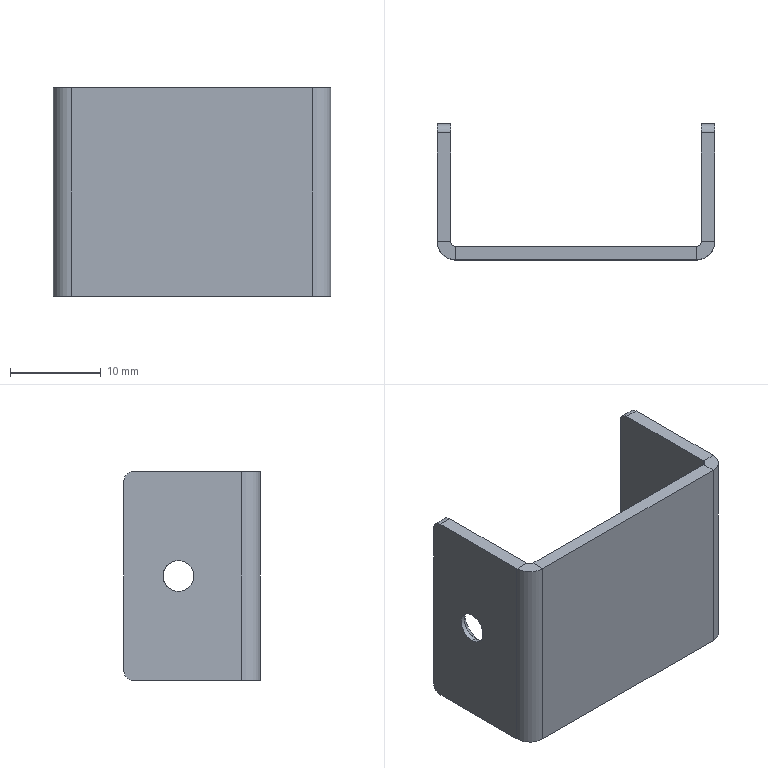Part | NX | features solid 2 | 1 solid | 34 faces | box 30.6 x 15 x 23 mm | volume 1909 mm3 | plane 18 | cylinder 12 | cone 4 | commonest cylinder face diameters 2 x4 3.4 x4 1 x2 4 x2
STEP:
#1=CARTESIAN_POINT('',(15.6,17.1,-1064.01));
#2=VERTEX_POINT('',#1);
#3=CARTESIAN_POINT('',(15.6,17.1,-1085.01));
#4=VERTEX_POINT('',#3);
#5=CARTESIAN_POINT('',(15.6,17.1,-1064.01));
#6=DIRECTION('',(0.,0.,-1.));
#7=VECTOR('',#6,1000.);
#8=LINE('',#5,#7);
#9=EDGE_CURVE('',#2,#4,#8,.T.);
#10=ORIENTED_EDGE('',*,*,#9,.F.);
#11=CARTESIAN_POINT('',(15.6,16.1,-1063.01));
#12=VERTEX_POINT('',#11);
#13=CARTESIAN_POINT('',(15.6,16.1,-1064.01));
#14=DIRECTION('',(-1.,0.,0.));
#15=DIRECTION('',(0.,0.,1.));
#16=AXIS2_PLACEMENT_3D('',#13,#14,#15);
#17=CIRCLE('',#16,1.);
#18=EDGE_CURVE('',#12,#2,#17,.T.);
#19=ORIENTED_EDGE('',*,*,#18,.F.);
#20=CARTESIAN_POINT('',(15.6,4.1,-1063.01));
#21=VERTEX_POINT('',#20);
#22=CARTESIAN_POINT('',(15.6,16.1,-1063.01));
#23=DIRECTION('',(0.,-1.,0.));
#24=VECTOR('',#23,1000.);
#25=LINE('',#22,#24);
#26=EDGE_CURVE('',#12,#21,#25,.T.);
#27=ORIENTED_EDGE('',*,*,#26,.T.);
#28=CARTESIAN_POINT('',(15.6,4.1,-1086.01));
#29=VERTEX_POINT('',#28);
#30=CARTESIAN_POINT('',(15.6,4.1,-1063.01));
#31=DIRECTION('',(0.,0.,-1.));
#32=VECTOR('',#31,1000.);
#33=LINE('',#30,#32);
#34=EDGE_CURVE('',#21,#29,#33,.T.);
#35=ORIENTED_EDGE('',*,*,#34,.T.);
#36=CARTESIAN_POINT('',(15.6,16.1,-1086.01));
#37=VERTEX_POINT('',#36);
#38=CARTESIAN_POINT('',(15.6,16.1,-1086.01));
#39=DIRECTION('',(0.,-1.,0.));
#40=VECTOR('',#39,1000.);
#41=LINE('',#38,#40);
#42=EDGE_CURVE('',#37,#29,#41,.T.);
#43=ORIENTED_EDGE('',*,*,#42,.F.);
#44=CARTESIAN_POINT('',(15.6,16.1,-1085.01));
#45=DIRECTION('',(-1.,0.,0.));
#46=DIRECTION('',(0.,1.,0.));
#47=AXIS2_PLACEMENT_3D('',#44,#45,#46);
#48=CIRCLE('',#47,1.);
#49=EDGE_CURVE('',#4,#37,#48,.T.);
#50=ORIENTED_EDGE('',*,*,#49,.F.);
#51=EDGE_LOOP('',(#10,#19,#27,#35,#43,#50));
#52=FACE_BOUND('',#51,.T.);
#53=CARTESIAN_POINT('',(15.6,11.1,-1076.21));
#54=VERTEX_POINT('',#53);
#55=CARTESIAN_POINT('',(15.6,11.1,-1072.81));
#56=VERTEX_POINT('',#55);
#57=CARTESIAN_POINT('',(15.6,11.1,-1074.51));
#58=DIRECTION('',(1.,0.,0.));
#59=DIRECTION('',(0.,0.,-1.));
#60=AXIS2_PLACEMENT_3D('',#57,#58,#59);
#61=CIRCLE('',#60,1.7);
#62=EDGE_CURVE('',#54,#56,#61,.T.);
#63=ORIENTED_EDGE('',*,*,#62,.F.);
#64=CARTESIAN_POINT('',(15.6,11.1,-1074.51));
#65=DIRECTION('',(1.,0.,0.));
#66=DIRECTION('',(0.,0.,1.));
#67=AXIS2_PLACEMENT_3D('',#64,#65,#66);
#68=CIRCLE('',#67,1.7);
#69=EDGE_CURVE('',#56,#54,#68,.T.);
#70=ORIENTED_EDGE('',*,*,#69,.F.);
#71=EDGE_LOOP('',(#63,#70));
#72=FACE_BOUND('',#71,.T.);
#73=CARTESIAN_POINT('',(15.6,2.1,-1086.01));
#74=DIRECTION('',(1.,0.,0.));
#75=DIRECTION('',(0.,-1.,0.));
#76=AXIS2_PLACEMENT_3D('',#73,#74,#75);
#77=PLANE('',#76);
#78=ADVANCED_FACE('',(#52,#72),#77,.T.);
#79=CARTESIAN_POINT('',(14.1,16.1,-1086.01));
#80=VERTEX_POINT('',#79);
#81=CARTESIAN_POINT('',(14.1,16.1,-1086.01));
#82=DIRECTION('',(1.,0.,0.));
#83=VECTOR('',#82,1000.);
#84=LINE('',#81,#83);
#85=EDGE_CURVE('',#80,#37,#84,.T.);
#86=ORIENTED_EDGE('',*,*,#85,.F.);
#87=CARTESIAN_POINT('',(14.1,17.1,-1085.01));
#88=VERTEX_POINT('',#87);
#89=CARTESIAN_POINT('',(14.1,16.1,-1085.01));
#90=DIRECTION('',(1.,0.,0.));
#91=DIRECTION('',(0.,0.,-1.));
#92=AXIS2_PLACEMENT_3D('',#89,#90,#91);
#93=CIRCLE('',#92,1.);
#94=EDGE_CURVE('',#80,#88,#93,.T.);
#95=ORIENTED_EDGE('',*,*,#94,.T.);
#96=CARTESIAN_POINT('',(15.6,17.1,-1085.01));
#97=DIRECTION('',(-1.,0.,0.));
#98=VECTOR('',#97,1000.);
#99=LINE('',#96,#98);
#100=EDGE_CURVE('',#4,#88,#99,.T.);
#101=ORIENTED_EDGE('',*,*,#100,.F.);
#102=ORIENTED_EDGE('',*,*,#49,.T.);
#103=EDGE_LOOP('',(#86,#95,#101,#102));
#104=FACE_BOUND('',#103,.T.);
#105=CARTESIAN_POINT('',(-54.89,16.1,-1085.01));
#106=DIRECTION('',(1.,0.,0.));
#107=DIRECTION('',(0.,0.,1.));
#108=AXIS2_PLACEMENT_3D('',#105,#106,#107);
#109=CYLINDRICAL_SURFACE('',#108,1.);
#110=ADVANCED_FACE('',(#104),#109,.T.);
#111=CARTESIAN_POINT('',(14.1,17.1,-1064.01));
#112=VERTEX_POINT('',#111);
#113=CARTESIAN_POINT('',(14.1,17.1,-1064.01));
#114=DIRECTION('',(0.,0.,-1.));
#115=VECTOR('',#114,1000.);
#116=LINE('',#113,#115);
#117=EDGE_CURVE('',#112,#88,#116,.T.);
#118=ORIENTED_EDGE('',*,*,#117,.F.);
#119=CARTESIAN_POINT('',(14.1,17.1,-1064.01));
#120=DIRECTION('',(1.,0.,0.));
#121=VECTOR('',#120,1000.);
#122=LINE('',#119,#121);
#123=EDGE_CURVE('',#112,#2,#122,.T.);
#124=ORIENTED_EDGE('',*,*,#123,.T.);
#125=ORIENTED_EDGE('',*,*,#9,.T.);
#126=ORIENTED_EDGE('',*,*,#100,.T.);
#127=EDGE_LOOP('',(#118,#124,#125,#126));
#128=FACE_BOUND('',#127,.T.);
#129=CARTESIAN_POINT('',(14.85,17.1,-1074.51));
#130=DIRECTION('',(0.,1.,0.));
#131=DIRECTION('',(0.,0.,-1.));
#132=AXIS2_PLACEMENT_3D('',#129,#130,#131);
#133=PLANE('',#132);
#134=ADVANCED_FACE('',(#128),#133,.T.);
#135=ORIENTED_EDGE('',*,*,#123,.F.);
#136=CARTESIAN_POINT('',(14.1,16.1,-1063.01));
#137=VERTEX_POINT('',#136);
#138=CARTESIAN_POINT('',(14.1,16.1,-1064.01));
#139=DIRECTION('',(1.,0.,0.));
#140=DIRECTION('',(0.,1.,0.));
#141=AXIS2_PLACEMENT_3D('',#138,#139,#140);
#142=CIRCLE('',#141,1.);
#143=EDGE_CURVE('',#112,#137,#142,.T.);
#144=ORIENTED_EDGE('',*,*,#143,.T.);
#145=CARTESIAN_POINT('',(15.6,16.1,-1063.01));
#146=DIRECTION('',(-1.,0.,0.));
#147=VECTOR('',#146,1000.);
#148=LINE('',#145,#147);
#149=EDGE_CURVE('',#12,#137,#148,.T.);
#150=ORIENTED_EDGE('',*,*,#149,.F.);
#151=ORIENTED_EDGE('',*,*,#18,.T.);
#152=EDGE_LOOP('',(#135,#144,#150,#151));
#153=FACE_BOUND('',#152,.T.);
#154=CARTESIAN_POINT('',(-54.259,16.1,-1064.01));
#155=DIRECTION('',(1.,0.,0.));
#156=DIRECTION('',(0.,-1.,0.));
#157=AXIS2_PLACEMENT_3D('',#154,#155,#156);
#158=CYLINDRICAL_SURFACE('',#157,1.);
#159=ADVANCED_FACE('',(#153),#158,.T.);
#160=CARTESIAN_POINT('',(14.1,4.1,-1063.01));
#161=VERTEX_POINT('',#160);
#162=CARTESIAN_POINT('',(14.1,16.1,-1063.01));
#163=DIRECTION('',(0.,-1.,0.));
#164=VECTOR('',#163,1000.);
#165=LINE('',#162,#164);
#166=EDGE_CURVE('',#137,#161,#165,.T.);
#167=ORIENTED_EDGE('',*,*,#166,.T.);
#168=CARTESIAN_POINT('',(14.1,4.1,-1063.01));
#169=DIRECTION('',(1.,0.,0.));
#170=VECTOR('',#169,1000.);
#171=LINE('',#168,#170);
#172=EDGE_CURVE('',#161,#21,#171,.T.);
#173=ORIENTED_EDGE('',*,*,#172,.T.);
#174=ORIENTED_EDGE('',*,*,#26,.F.);
#175=ORIENTED_EDGE('',*,*,#149,.T.);
#176=EDGE_LOOP('',(#167,#173,#174,#175));
#177=FACE_BOUND('',#176,.T.);
#178=CARTESIAN_POINT('',(14.85,9.975,-1063.01));
#179=DIRECTION('',(0.,0.,-1.));
#180=DIRECTION('',(0.,-1.,0.));
#181=AXIS2_PLACEMENT_3D('',#178,#179,#180);
#182=PLANE('',#181);
#183=ADVANCED_FACE('',(#177),#182,.F.);
#184=ORIENTED_EDGE('',*,*,#172,.F.);
#185=CARTESIAN_POINT('',(13.6,3.6,-1063.01));
#186=VERTEX_POINT('',#185);
#187=CARTESIAN_POINT('',(13.6,4.1,-1063.01));
#188=DIRECTION('',(0.,0.,1.));
#189=DIRECTION('',(0.,-1.,0.));
#190=AXIS2_PLACEMENT_3D('',#187,#188,#189);
#191=CIRCLE('',#190,0.5);
#192=EDGE_CURVE('',#186,#161,#191,.T.);
#193=ORIENTED_EDGE('',*,*,#192,.F.);
#194=CARTESIAN_POINT('',(13.6,2.1,-1063.01));
#195=VERTEX_POINT('',#194);
#196=CARTESIAN_POINT('',(13.6,3.6,-1063.01));
#197=DIRECTION('',(0.,-1.,0.));
#198=VECTOR('',#197,1000.);
#199=LINE('',#196,#198);
#200=EDGE_CURVE('',#186,#195,#199,.T.);
#201=ORIENTED_EDGE('',*,*,#200,.T.);
#202=CARTESIAN_POINT('',(13.6,4.1,-1063.01));
#203=DIRECTION('',(0.,0.,-1.));
#204=DIRECTION('',(1.,0.,0.));
#205=AXIS2_PLACEMENT_3D('',#202,#203,#204);
#206=CIRCLE('',#205,2.);
#207=EDGE_CURVE('',#21,#195,#206,.T.);
#208=ORIENTED_EDGE('',*,*,#207,.F.);
#209=EDGE_LOOP('',(#184,#193,#201,#208));
#210=FACE_BOUND('',#209,.T.);
#211=CARTESIAN_POINT('',(14.484,3.216,-1063.01));
#212=DIRECTION('',(0.,0.,-1.));
#213=DIRECTION('',(-1.,0.,0.));
#214=AXIS2_PLACEMENT_3D('',#211,#212,#213);
#215=PLANE('',#214);
#216=ADVANCED_FACE('',(#210),#215,.F.);
#217=CARTESIAN_POINT('',(13.6,2.1,-1086.01));
#218=VERTEX_POINT('',#217);
#219=CARTESIAN_POINT('',(13.6,4.1,-1086.01));
#220=DIRECTION('',(0.,0.,1.));
#221=DIRECTION('',(0.,-1.,0.));
#222=AXIS2_PLACEMENT_3D('',#219,#220,#221);
#223=CIRCLE('',#222,2.);
#224=EDGE_CURVE('',#218,#29,#223,.T.);
#225=ORIENTED_EDGE('',*,*,#224,.T.);
#226=ORIENTED_EDGE('',*,*,#34,.F.);
#227=ORIENTED_EDGE('',*,*,#207,.T.);
#228=CARTESIAN_POINT('',(13.6,2.1,-1086.01));
#229=DIRECTION('',(0.,0.,1.));
#230=VECTOR('',#229,1000.);
#231=LINE('',#228,#230);
#232=EDGE_CURVE('',#218,#195,#231,.T.);
#233=ORIENTED_EDGE('',*,*,#232,.F.);
#234=EDGE_LOOP('',(#225,#226,#227,#233));
#235=FACE_BOUND('',#234,.T.);
#236=CARTESIAN_POINT('',(13.6,4.1,-1019.945));
#237=DIRECTION('',(0.,0.,-1.));
#238=DIRECTION('',(-1.,0.,0.));
#239=AXIS2_PLACEMENT_3D('',#236,#237,#238);
#240=CYLINDRICAL_SURFACE('',#239,2.);
#241=ADVANCED_FACE('',(#235),#240,.T.);
#242=CARTESIAN_POINT('',(-13.,2.1,-1063.01));
#243=VERTEX_POINT('',#242);
#244=CARTESIAN_POINT('',(13.6,2.1,-1063.01));
#245=DIRECTION('',(-1.,0.,0.));
#246=VECTOR('',#245,1000.);
#247=LINE('',#244,#246);
#248=EDGE_CURVE('',#195,#243,#247,.T.);
#249=ORIENTED_EDGE('',*,*,#248,.T.);
#250=CARTESIAN_POINT('',(-13.,2.1,-1086.01));
#251=VERTEX_POINT('',#250);
#252=CARTESIAN_POINT('',(-13.,2.1,-1063.01));
#253=DIRECTION('',(0.,0.,-1.));
#254=VECTOR('',#253,1000.);
#255=LINE('',#252,#254);
#256=EDGE_CURVE('',#243,#251,#255,.T.);
#257=ORIENTED_EDGE('',*,*,#256,.T.);
#258=CARTESIAN_POINT('',(13.6,2.1,-1086.01));
#259=DIRECTION('',(-1.,0.,0.));
#260=VECTOR('',#259,1000.);
#261=LINE('',#258,#260);
#262=EDGE_CURVE('',#218,#251,#261,.T.);
#263=ORIENTED_EDGE('',*,*,#262,.F.);
#264=ORIENTED_EDGE('',*,*,#232,.T.);
#265=EDGE_LOOP('',(#249,#257,#263,#264));
#266=FACE_BOUND('',#265,.T.);
#267=CARTESIAN_POINT('',(-15.,2.1,-1086.01));
#268=DIRECTION('',(0.,-1.,0.));
#269=DIRECTION('',(-1.,0.,0.));
#270=AXIS2_PLACEMENT_3D('',#267,#268,#269);
#271=PLANE('',#270);
#272=ADVANCED_FACE('',(#266),#271,.T.);
#273=ORIENTED_EDGE('',*,*,#262,.T.);
#274=CARTESIAN_POINT('',(-13.,3.6,-1086.01));
#275=VERTEX_POINT('',#274);
#276=CARTESIAN_POINT('',(-13.,3.6,-1086.01));
#277=DIRECTION('',(0.,-1.,0.));
#278=VECTOR('',#277,1000.);
#279=LINE('',#276,#278);
#280=EDGE_CURVE('',#275,#251,#279,.T.);
#281=ORIENTED_EDGE('',*,*,#280,.F.);
#282=CARTESIAN_POINT('',(13.6,3.6,-1086.01));
#283=VERTEX_POINT('',#282);
#284=CARTESIAN_POINT('',(13.6,3.6,-1086.01));
#285=DIRECTION('',(-1.,0.,0.));
#286=VECTOR('',#285,1000.);
#287=LINE('',#284,#286);
#288=EDGE_CURVE('',#283,#275,#287,.T.);
#289=ORIENTED_EDGE('',*,*,#288,.F.);
#290=CARTESIAN_POINT('',(13.6,3.6,-1086.01));
#291=DIRECTION('',(0.,-1.,0.));
#292=VECTOR('',#291,1000.);
#293=LINE('',#290,#292);
#294=EDGE_CURVE('',#283,#218,#293,.T.);
#295=ORIENTED_EDGE('',*,*,#294,.T.);
#296=EDGE_LOOP('',(#273,#281,#289,#295));
#297=FACE_BOUND('',#296,.T.);
#298=CARTESIAN_POINT('',(0.3,2.85,-1086.01));
#299=DIRECTION('',(0.,0.,-1.));
#300=DIRECTION('',(-1.,0.,0.));
#301=AXIS2_PLACEMENT_3D('',#298,#299,#300);
#302=PLANE('',#301);
#303=ADVANCED_FACE('',(#297),#302,.T.);
#304=ORIENTED_EDGE('',*,*,#294,.F.);
#305=CARTESIAN_POINT('',(14.1,4.1,-1086.01));
#306=VERTEX_POINT('',#305);
#307=CARTESIAN_POINT('',(13.6,4.1,-1086.01));
#308=DIRECTION('',(0.,0.,-1.));
#309=DIRECTION('',(1.,0.,0.));
#310=AXIS2_PLACEMENT_3D('',#307,#308,#309);
#311=CIRCLE('',#310,0.5);
#312=EDGE_CURVE('',#306,#283,#311,.T.);
#313=ORIENTED_EDGE('',*,*,#312,.F.);
#314=CARTESIAN_POINT('',(14.1,4.1,-1086.01));
#315=DIRECTION('',(1.,0.,0.));
#316=VECTOR('',#315,1000.);
#317=LINE('',#314,#316);
#318=EDGE_CURVE('',#306,#29,#317,.T.);
#319=ORIENTED_EDGE('',*,*,#318,.T.);
#320=ORIENTED_EDGE('',*,*,#224,.F.);
#321=EDGE_LOOP('',(#304,#313,#319,#320));
#322=FACE_BOUND('',#321,.T.);
#323=CARTESIAN_POINT('',(14.484,3.216,-1086.01));
#324=DIRECTION('',(0.,0.,1.));
#325=DIRECTION('',(0.,1.,0.));
#326=AXIS2_PLACEMENT_3D('',#323,#324,#325);
#327=PLANE('',#326);
#328=ADVANCED_FACE('',(#322),#327,.F.);
#329=ORIENTED_EDGE('',*,*,#42,.T.);
#330=ORIENTED_EDGE('',*,*,#318,.F.);
#331=CARTESIAN_POINT('',(14.1,16.1,-1086.01));
#332=DIRECTION('',(0.,-1.,0.));
#333=VECTOR('',#332,1000.);
#334=LINE('',#331,#333);
#335=EDGE_CURVE('',#80,#306,#334,.T.);
#336=ORIENTED_EDGE('',*,*,#335,.F.);
#337=ORIENTED_EDGE('',*,*,#85,.T.);
#338=EDGE_LOOP('',(#329,#330,#336,#337));
#339=FACE_BOUND('',#338,.T.);
#340=CARTESIAN_POINT('',(14.85,9.975,-1086.01));
#341=DIRECTION('',(0.,0.,-1.));
#342=DIRECTION('',(0.,-1.,0.));
#343=AXIS2_PLACEMENT_3D('',#340,#341,#342);
#344=PLANE('',#343);
#345=ADVANCED_FACE('',(#339),#344,.T.);
#346=ORIENTED_EDGE('',*,*,#335,.T.);
#347=CARTESIAN_POINT('',(14.1,4.1,-1086.01));
#348=DIRECTION('',(0.,0.,1.));
#349=VECTOR('',#348,1000.);
#350=LINE('',#347,#349);
#351=EDGE_CURVE('',#306,#161,#350,.T.);
#352=ORIENTED_EDGE('',*,*,#351,.T.);
#353=ORIENTED_EDGE('',*,*,#166,.F.);
#354=ORIENTED_EDGE('',*,*,#143,.F.);
#355=ORIENTED_EDGE('',*,*,#117,.T.);
#356=ORIENTED_EDGE('',*,*,#94,.F.);
#357=EDGE_LOOP('',(#346,#352,#353,#354,#355,#356));
#358=FACE_BOUND('',#357,.T.);
#359=CARTESIAN_POINT('',(14.1,8.4,-1074.51));
#360=VERTEX_POINT('',#359);
#361=CARTESIAN_POINT('',(14.1,11.1,-1071.81));
#362=VERTEX_POINT('',#361);
#363=CARTESIAN_POINT('',(14.1,11.1,-1074.51));
#364=DIRECTION('',(-1.,0.,0.));
#365=DIRECTION('',(0.,-1.,0.));
#366=AXIS2_PLACEMENT_3D('',#363,#364,#365);
#367=CIRCLE('',#366,2.7);
#368=EDGE_CURVE('',#360,#362,#367,.T.);
#369=ORIENTED_EDGE('',*,*,#368,.F.);
#370=CARTESIAN_POINT('',(14.1,11.1,-1077.21));
#371=VERTEX_POINT('',#370);
#372=CARTESIAN_POINT('',(14.1,11.1,-1074.51));
#373=DIRECTION('',(-1.,0.,0.));
#374=DIRECTION('',(0.,0.,-1.));
#375=AXIS2_PLACEMENT_3D('',#372,#373,#374);
#376=CIRCLE('',#375,2.7);
#377=EDGE_CURVE('',#371,#360,#376,.T.);
#378=ORIENTED_EDGE('',*,*,#377,.F.);
#379=CARTESIAN_POINT('',(14.1,13.8,-1074.51));
#380=VERTEX_POINT('',#379);
#381=CARTESIAN_POINT('',(14.1,11.1,-1074.51));
#382=DIRECTION('',(-1.,0.,0.));
#383=DIRECTION('',(0.,1.,0.));
#384=AXIS2_PLACEMENT_3D('',#381,#382,#383);
#385=CIRCLE('',#384,2.7);
#386=EDGE_CURVE('',#380,#371,#385,.T.);
#387=ORIENTED_EDGE('',*,*,#386,.F.);
#388=CARTESIAN_POINT('',(14.1,11.1,-1074.51));
#389=DIRECTION('',(-1.,0.,0.));
#390=DIRECTION('',(0.,0.,1.));
#391=AXIS2_PLACEMENT_3D('',#388,#389,#390);
#392=CIRCLE('',#391,2.7);
#393=EDGE_CURVE('',#362,#380,#392,.T.);
#394=ORIENTED_EDGE('',*,*,#393,.F.);
#395=EDGE_LOOP('',(#369,#378,#387,#394));
#396=FACE_BOUND('',#395,.T.);
#397=CARTESIAN_POINT('',(14.1,2.1,-1086.01));
#398=DIRECTION('',(1.,0.,0.));
#399=DIRECTION('',(0.,-1.,0.));
#400=AXIS2_PLACEMENT_3D('',#397,#398,#399);
#401=PLANE('',#400);
#402=ADVANCED_FACE('',(#358,#396),#401,.F.);
#403=ORIENTED_EDGE('',*,*,#192,.T.);
#404=ORIENTED_EDGE('',*,*,#351,.F.);
#405=ORIENTED_EDGE('',*,*,#312,.T.);
#406=CARTESIAN_POINT('',(13.6,3.6,-1063.01));
#407=DIRECTION('',(0.,0.,-1.));
#408=VECTOR('',#407,1000.);
#409=LINE('',#406,#408);
#410=EDGE_CURVE('',#186,#283,#409,.T.);
#411=ORIENTED_EDGE('',*,*,#410,.F.);
#412=EDGE_LOOP('',(#403,#404,#405,#411));
#413=FACE_BOUND('',#412,.T.);
#414=CARTESIAN_POINT('',(13.6,4.1,-1019.945));
#415=DIRECTION('',(0.,0.,-1.));
#416=DIRECTION('',(-1.,0.,0.));
#417=AXIS2_PLACEMENT_3D('',#414,#415,#416);
#418=CYLINDRICAL_SURFACE('',#417,0.5);
#419=ADVANCED_FACE('',(#413),#418,.F.);
#420=ORIENTED_EDGE('',*,*,#288,.T.);
#421=CARTESIAN_POINT('',(-13.,3.6,-1063.01));
#422=VERTEX_POINT('',#421);
#423=CARTESIAN_POINT('',(-13.,3.6,-1086.01));
#424=DIRECTION('',(0.,0.,1.));
#425=VECTOR('',#424,1000.);
#426=LINE('',#423,#425);
#427=EDGE_CURVE('',#275,#422,#426,.T.);
#428=ORIENTED_EDGE('',*,*,#427,.T.);
#429=CARTESIAN_POINT('',(13.6,3.6,-1063.01));
#430=DIRECTION('',(-1.,0.,0.));
#431=VECTOR('',#430,1000.);
#432=LINE('',#429,#431);
#433=EDGE_CURVE('',#186,#422,#432,.T.);
#434=ORIENTED_EDGE('',*,*,#433,.F.);
#435=ORIENTED_EDGE('',*,*,#410,.T.);
#436=EDGE_LOOP('',(#420,#428,#434,#435));
#437=FACE_BOUND('',#436,.T.);
#438=CARTESIAN_POINT('',(-15.,3.6,-1086.01));
#439=DIRECTION('',(0.,-1.,0.));
#440=DIRECTION('',(-1.,0.,0.));
#441=AXIS2_PLACEMENT_3D('',#438,#439,#440);
#442=PLANE('',#441);
#443=ADVANCED_FACE('',(#437),#442,.F.);
#444=ORIENTED_EDGE('',*,*,#248,.F.);
#445=ORIENTED_EDGE('',*,*,#200,.F.);
#446=ORIENTED_EDGE('',*,*,#433,.T.);
#447=CARTESIAN_POINT('',(-13.,3.6,-1063.01));
#448=DIRECTION('',(0.,-1.,0.));
#449=VECTOR('',#448,1000.);
#450=LINE('',#447,#449);
#451=EDGE_CURVE('',#422,#243,#450,.T.);
#452=ORIENTED_EDGE('',*,*,#451,.T.);
#453=EDGE_LOOP('',(#444,#445,#446,#452));
#454=FACE_BOUND('',#453,.T.);
#455=CARTESIAN_POINT('',(0.3,2.85,-1063.01));
#456=DIRECTION('',(0.,0.,-1.));
#457=DIRECTION('',(-1.,0.,0.));
#458=AXIS2_PLACEMENT_3D('',#455,#456,#457);
#459=PLANE('',#458);
#460=ADVANCED_FACE('',(#454),#459,.F.);
#461=ORIENTED_EDGE('',*,*,#451,.F.);
#462=CARTESIAN_POINT('',(-13.5,4.1,-1063.01));
#463=VERTEX_POINT('',#462);
#464=CARTESIAN_POINT('',(-13.,4.1,-1063.01));
#465=DIRECTION('',(0.,0.,1.));
#466=DIRECTION('',(-1.,0.,0.));
#467=AXIS2_PLACEMENT_3D('',#464,#465,#466);
#468=CIRCLE('',#467,0.5);
#469=EDGE_CURVE('',#463,#422,#468,.T.);
#470=ORIENTED_EDGE('',*,*,#469,.F.);
#471=CARTESIAN_POINT('',(-15.,4.1,-1063.01));
#472=VERTEX_POINT('',#471);
#473=CARTESIAN_POINT('',(-13.5,4.1,-1063.01));
#474=DIRECTION('',(-1.,0.,0.));
#475=VECTOR('',#474,1000.);
#476=LINE('',#473,#475);
#477=EDGE_CURVE('',#463,#472,#476,.T.);
#478=ORIENTED_EDGE('',*,*,#477,.T.);
#479=CARTESIAN_POINT('',(-13.,4.1,-1063.01));
#480=DIRECTION('',(0.,0.,-1.));
#481=DIRECTION('',(0.,-1.,0.));
#482=AXIS2_PLACEMENT_3D('',#479,#480,#481);
#483=CIRCLE('',#482,2.);
#484=EDGE_CURVE('',#243,#472,#483,.T.);
#485=ORIENTED_EDGE('',*,*,#484,.F.);
#486=EDGE_LOOP('',(#461,#470,#478,#485));
#487=FACE_BOUND('',#486,.T.);
#488=CARTESIAN_POINT('',(-13.884,3.216,-1063.01));
#489=DIRECTION('',(0.,0.,-1.));
#490=DIRECTION('',(0.,1.,0.));
#491=AXIS2_PLACEMENT_3D('',#488,#489,#490);
#492=PLANE('',#491);
#493=ADVANCED_FACE('',(#487),#492,.F.);
#494=CARTESIAN_POINT('',(-15.,4.1,-1086.01));
#495=VERTEX_POINT('',#494);
#496=CARTESIAN_POINT('',(-13.,4.1,-1086.01));
#497=DIRECTION('',(0.,0.,1.));
#498=DIRECTION('',(-1.,0.,0.));
#499=AXIS2_PLACEMENT_3D('',#496,#497,#498);
#500=CIRCLE('',#499,2.);
#501=EDGE_CURVE('',#495,#251,#500,.T.);
#502=ORIENTED_EDGE('',*,*,#501,.T.);
#503=ORIENTED_EDGE('',*,*,#256,.F.);
#504=ORIENTED_EDGE('',*,*,#484,.T.);
#505=CARTESIAN_POINT('',(-15.,4.1,-1086.01));
#506=DIRECTION('',(0.,0.,1.));
#507=VECTOR('',#506,1000.);
#508=LINE('',#505,#507);
#509=EDGE_CURVE('',#495,#472,#508,.T.);
#510=ORIENTED_EDGE('',*,*,#509,.F.);
#511=EDGE_LOOP('',(#502,#503,#504,#510));
#512=FACE_BOUND('',#511,.T.);
#513=CARTESIAN_POINT('',(-13.,4.1,-1019.945));
#514=DIRECTION('',(0.,0.,-1.));
#515=DIRECTION('',(0.,1.,0.));
#516=AXIS2_PLACEMENT_3D('',#513,#514,#515);
#517=CYLINDRICAL_SURFACE('',#516,2.);
#518=ADVANCED_FACE('',(#512),#517,.T.);
#519=CARTESIAN_POINT('',(-15.,16.1,-1086.01));
#520=VERTEX_POINT('',#519);
#521=CARTESIAN_POINT('',(-15.,4.1,-1086.01));
#522=DIRECTION('',(0.,1.,0.));
#523=VECTOR('',#522,1000.);
#524=LINE('',#521,#523);
#525=EDGE_CURVE('',#495,#520,#524,.T.);
#526=ORIENTED_EDGE('',*,*,#525,.F.);
#527=ORIENTED_EDGE('',*,*,#509,.T.);
#528=CARTESIAN_POINT('',(-15.,16.1,-1063.01));
#529=VERTEX_POINT('',#528);
#530=CARTESIAN_POINT('',(-15.,4.1,-1063.01));
#531=DIRECTION('',(0.,1.,0.));
#532=VECTOR('',#531,1000.);
#533=LINE('',#530,#532);
#534=EDGE_CURVE('',#472,#529,#533,.T.);
#535=ORIENTED_EDGE('',*,*,#534,.T.);
#536=CARTESIAN_POINT('',(-15.,17.1,-1064.01));
#537=VERTEX_POINT('',#536);
#538=CARTESIAN_POINT('',(-15.,16.1,-1064.01));
#539=DIRECTION('',(1.,0.,0.));
#540=DIRECTION('',(0.,1.,0.));
#541=AXIS2_PLACEMENT_3D('',#538,#539,#540);
#542=CIRCLE('',#541,1.);
#543=EDGE_CURVE('',#537,#529,#542,.T.);
#544=ORIENTED_EDGE('',*,*,#543,.F.);
#545=CARTESIAN_POINT('',(-15.,17.1,-1085.01));
#546=VERTEX_POINT('',#545);
#547=CARTESIAN_POINT('',(-15.,17.1,-1064.01));
#548=DIRECTION('',(0.,0.,-1.));
#549=VECTOR('',#548,1000.);
#550=LINE('',#547,#549);
#551=EDGE_CURVE('',#537,#546,#550,.T.);
#552=ORIENTED_EDGE('',*,*,#551,.T.);
#553=CARTESIAN_POINT('',(-15.,16.1,-1085.01));
#554=DIRECTION('',(1.,0.,0.));
#555=DIRECTION('',(0.,0.,-1.));
#556=AXIS2_PLACEMENT_3D('',#553,#554,#555);
#557=CIRCLE('',#556,1.);
#558=EDGE_CURVE('',#520,#546,#557,.T.);
#559=ORIENTED_EDGE('',*,*,#558,.F.);
#560=EDGE_LOOP('',(#526,#527,#535,#544,#552,#559));
#561=FACE_BOUND('',#560,.T.);
#562=CARTESIAN_POINT('',(-15.,11.1,-1072.81));
#563=VERTEX_POINT('',#562);
#564=CARTESIAN_POINT('',(-15.,11.1,-1076.21));
#565=VERTEX_POINT('',#564);
#566=CARTESIAN_POINT('',(-15.,11.1,-1074.51));
#567=DIRECTION('',(-1.,0.,0.));
#568=DIRECTION('',(0.,0.,1.));
#569=AXIS2_PLACEMENT_3D('',#566,#567,#568);
#570=CIRCLE('',#569,1.7);
#571=EDGE_CURVE('',#563,#565,#570,.T.);
#572=ORIENTED_EDGE('',*,*,#571,.F.);
#573=CARTESIAN_POINT('',(-15.,11.1,-1074.51));
#574=DIRECTION('',(-1.,0.,0.));
#575=DIRECTION('',(0.,0.,-1.));
#576=AXIS2_PLACEMENT_3D('',#573,#574,#575);
#577=CIRCLE('',#576,1.7);
#578=EDGE_CURVE('',#565,#563,#577,.T.);
#579=ORIENTED_EDGE('',*,*,#578,.F.);
#580=EDGE_LOOP('',(#572,#579));
#581=FACE_BOUND('',#580,.T.);
#582=CARTESIAN_POINT('',(-15.,17.1,-1086.01));
#583=DIRECTION('',(-1.,0.,0.));
#584=DIRECTION('',(0.,1.,0.));
#585=AXIS2_PLACEMENT_3D('',#582,#583,#584);
#586=PLANE('',#585);
#587=ADVANCED_FACE('',(#561,#581),#586,.T.);
#588=CARTESIAN_POINT('',(-13.5,17.1,-1085.01));
#589=VERTEX_POINT('',#588);
#590=CARTESIAN_POINT('',(-13.5,17.1,-1085.01));
#591=DIRECTION('',(-1.,0.,0.));
#592=VECTOR('',#591,1000.);
#593=LINE('',#590,#592);
#594=EDGE_CURVE('',#589,#546,#593,.T.);
#595=ORIENTED_EDGE('',*,*,#594,.F.);
#596=CARTESIAN_POINT('',(-13.5,16.1,-1086.01));
#597=VERTEX_POINT('',#596);
#598=CARTESIAN_POINT('',(-13.5,16.1,-1085.01));
#599=DIRECTION('',(-1.,0.,0.));
#600=DIRECTION('',(0.,1.,0.));
#601=AXIS2_PLACEMENT_3D('',#598,#599,#600);
#602=CIRCLE('',#601,1.);
#603=EDGE_CURVE('',#589,#597,#602,.T.);
#604=ORIENTED_EDGE('',*,*,#603,.T.);
#605=CARTESIAN_POINT('',(-15.,16.1,-1086.01));
#606=DIRECTION('',(1.,0.,0.));
#607=VECTOR('',#606,1000.);
#608=LINE('',#605,#607);
#609=EDGE_CURVE('',#520,#597,#608,.T.);
#610=ORIENTED_EDGE('',*,*,#609,.F.);
#611=ORIENTED_EDGE('',*,*,#558,.T.);
#612=EDGE_LOOP('',(#595,#604,#610,#611));
#613=FACE_BOUND('',#612,.T.);
#614=CARTESIAN_POINT('',(53.191,16.1,-1085.01));
#615=DIRECTION('',(-1.,0.,0.));
#616=DIRECTION('',(0.,-1.,0.));
#617=AXIS2_PLACEMENT_3D('',#614,#615,#616);
#618=CYLINDRICAL_SURFACE('',#617,1.);
#619=ADVANCED_FACE('',(#613),#618,.T.);
#620=CARTESIAN_POINT('',(-13.5,4.1,-1086.01));
#621=VERTEX_POINT('',#620);
#622=CARTESIAN_POINT('',(-13.5,4.1,-1086.01));
#623=DIRECTION('',(0.,1.,0.));
#624=VECTOR('',#623,1000.);
#625=LINE('',#622,#624);
#626=EDGE_CURVE('',#621,#597,#625,.T.);
#627=ORIENTED_EDGE('',*,*,#626,.F.);
#628=CARTESIAN_POINT('',(-13.5,4.1,-1086.01));
#629=DIRECTION('',(-1.,0.,0.));
#630=VECTOR('',#629,1000.);
#631=LINE('',#628,#630);
#632=EDGE_CURVE('',#621,#495,#631,.T.);
#633=ORIENTED_EDGE('',*,*,#632,.T.);
#634=ORIENTED_EDGE('',*,*,#525,.T.);
#635=ORIENTED_EDGE('',*,*,#609,.T.);
#636=EDGE_LOOP('',(#627,#633,#634,#635));
#637=FACE_BOUND('',#636,.T.);
#638=CARTESIAN_POINT('',(-14.25,9.975,-1086.01));
#639=DIRECTION('',(0.,0.,-1.));
#640=DIRECTION('',(0.,1.,0.));
#641=AXIS2_PLACEMENT_3D('',#638,#639,#640);
#642=PLANE('',#641);
#643=ADVANCED_FACE('',(#637),#642,.T.);
#644=ORIENTED_EDGE('',*,*,#632,.F.);
#645=CARTESIAN_POINT('',(-13.,4.1,-1086.01));
#646=DIRECTION('',(0.,0.,-1.));
#647=DIRECTION('',(0.,-1.,0.));
#648=AXIS2_PLACEMENT_3D('',#645,#646,#647);
#649=CIRCLE('',#648,0.5);
#650=EDGE_CURVE('',#275,#621,#649,.T.);
#651=ORIENTED_EDGE('',*,*,#650,.F.);
#652=ORIENTED_EDGE('',*,*,#280,.T.);
#653=ORIENTED_EDGE('',*,*,#501,.F.);
#654=EDGE_LOOP('',(#644,#651,#652,#653));
#655=FACE_BOUND('',#654,.T.);
#656=CARTESIAN_POINT('',(-13.884,3.216,-1086.01));
#657=DIRECTION('',(0.,0.,1.));
#658=DIRECTION('',(1.,0.,0.));
#659=AXIS2_PLACEMENT_3D('',#656,#657,#658);
#660=PLANE('',#659);
#661=ADVANCED_FACE('',(#655),#660,.F.);
#662=ORIENTED_EDGE('',*,*,#469,.T.);
#663=ORIENTED_EDGE('',*,*,#427,.F.);
#664=ORIENTED_EDGE('',*,*,#650,.T.);
#665=CARTESIAN_POINT('',(-13.5,4.1,-1063.01));
#666=DIRECTION('',(0.,0.,-1.));
#667=VECTOR('',#666,1000.);
#668=LINE('',#665,#667);
#669=EDGE_CURVE('',#463,#621,#668,.T.);
#670=ORIENTED_EDGE('',*,*,#669,.F.);
#671=EDGE_LOOP('',(#662,#663,#664,#670));
#672=FACE_BOUND('',#671,.T.);
#673=CARTESIAN_POINT('',(-13.,4.1,-1019.945));
#674=DIRECTION('',(0.,0.,-1.));
#675=DIRECTION('',(0.,1.,0.));
#676=AXIS2_PLACEMENT_3D('',#673,#674,#675);
#677=CYLINDRICAL_SURFACE('',#676,0.5);
#678=ADVANCED_FACE('',(#672),#677,.F.);
#679=CARTESIAN_POINT('',(-13.5,17.1,-1064.01));
#680=VERTEX_POINT('',#679);
#681=CARTESIAN_POINT('',(-13.5,17.1,-1064.01));
#682=DIRECTION('',(0.,0.,-1.));
#683=VECTOR('',#682,1000.);
#684=LINE('',#681,#683);
#685=EDGE_CURVE('',#680,#589,#684,.T.);
#686=ORIENTED_EDGE('',*,*,#685,.F.);
#687=CARTESIAN_POINT('',(-13.5,16.1,-1063.01));
#688=VERTEX_POINT('',#687);
#689=CARTESIAN_POINT('',(-13.5,16.1,-1064.01));
#690=DIRECTION('',(-1.,0.,0.));
#691=DIRECTION('',(0.,0.,1.));
#692=AXIS2_PLACEMENT_3D('',#689,#690,#691);
#693=CIRCLE('',#692,1.);
#694=EDGE_CURVE('',#688,#680,#693,.T.);
#695=ORIENTED_EDGE('',*,*,#694,.F.);
#696=CARTESIAN_POINT('',(-13.5,4.1,-1063.01));
#697=DIRECTION('',(0.,1.,0.));
#698=VECTOR('',#697,1000.);
#699=LINE('',#696,#698);
#700=EDGE_CURVE('',#463,#688,#699,.T.);
#701=ORIENTED_EDGE('',*,*,#700,.F.);
#702=ORIENTED_EDGE('',*,*,#669,.T.);
#703=ORIENTED_EDGE('',*,*,#626,.T.);
#704=ORIENTED_EDGE('',*,*,#603,.F.);
#705=EDGE_LOOP('',(#686,#695,#701,#702,#703,#704));
#706=FACE_BOUND('',#705,.T.);
#707=CARTESIAN_POINT('',(-13.5,8.4,-1074.51));
#708=VERTEX_POINT('',#707);
#709=CARTESIAN_POINT('',(-13.5,11.1,-1077.21));
#710=VERTEX_POINT('',#709);
#711=CARTESIAN_POINT('',(-13.5,11.1,-1074.51));
#712=DIRECTION('',(1.,0.,0.));
#713=DIRECTION('',(0.,-1.,0.));
#714=AXIS2_PLACEMENT_3D('',#711,#712,#713);
#715=CIRCLE('',#714,2.7);
#716=EDGE_CURVE('',#708,#710,#715,.T.);
#717=ORIENTED_EDGE('',*,*,#716,.F.);
#718=CARTESIAN_POINT('',(-13.5,11.1,-1071.81));
#719=VERTEX_POINT('',#718);
#720=CARTESIAN_POINT('',(-13.5,11.1,-1074.51));
#721=DIRECTION('',(1.,0.,0.));
#722=DIRECTION('',(0.,0.,1.));
#723=AXIS2_PLACEMENT_3D('',#720,#721,#722);
#724=CIRCLE('',#723,2.7);
#725=EDGE_CURVE('',#719,#708,#724,.T.);
#726=ORIENTED_EDGE('',*,*,#725,.F.);
#727=CARTESIAN_POINT('',(-13.5,13.8,-1074.51));
#728=VERTEX_POINT('',#727);
#729=CARTESIAN_POINT('',(-13.5,11.1,-1074.51));
#730=DIRECTION('',(1.,0.,0.));
#731=DIRECTION('',(0.,1.,0.));
#732=AXIS2_PLACEMENT_3D('',#729,#730,#731);
#733=CIRCLE('',#732,2.7);
#734=EDGE_CURVE('',#728,#719,#733,.T.);
#735=ORIENTED_EDGE('',*,*,#734,.F.);
#736=CARTESIAN_POINT('',(-13.5,11.1,-1074.51));
#737=DIRECTION('',(1.,0.,0.));
#738=DIRECTION('',(0.,0.,-1.));
#739=AXIS2_PLACEMENT_3D('',#736,#737,#738);
#740=CIRCLE('',#739,2.7);
#741=EDGE_CURVE('',#710,#728,#740,.T.);
#742=ORIENTED_EDGE('',*,*,#741,.F.);
#743=EDGE_LOOP('',(#717,#726,#735,#742));
#744=FACE_BOUND('',#743,.T.);
#745=CARTESIAN_POINT('',(-13.5,17.1,-1086.01));
#746=DIRECTION('',(-1.,0.,0.));
#747=DIRECTION('',(0.,1.,0.));
#748=AXIS2_PLACEMENT_3D('',#745,#746,#747);
#749=PLANE('',#748);
#750=ADVANCED_FACE('',(#706,#744),#749,.F.);
#751=ORIENTED_EDGE('',*,*,#534,.F.);
#752=ORIENTED_EDGE('',*,*,#477,.F.);
#753=ORIENTED_EDGE('',*,*,#700,.T.);
#754=CARTESIAN_POINT('',(-13.5,16.1,-1063.01));
#755=DIRECTION('',(-1.,0.,0.));
#756=VECTOR('',#755,1000.);
#757=LINE('',#754,#756);
#758=EDGE_CURVE('',#688,#529,#757,.T.);
#759=ORIENTED_EDGE('',*,*,#758,.T.);
#760=EDGE_LOOP('',(#751,#752,#753,#759));
#761=FACE_BOUND('',#760,.T.);
#762=CARTESIAN_POINT('',(-14.25,9.975,-1063.01));
#763=DIRECTION('',(0.,0.,-1.));
#764=DIRECTION('',(0.,1.,0.));
#765=AXIS2_PLACEMENT_3D('',#762,#763,#764);
#766=PLANE('',#765);
#767=ADVANCED_FACE('',(#761),#766,.F.);
#768=ORIENTED_EDGE('',*,*,#758,.F.);
#769=ORIENTED_EDGE('',*,*,#694,.T.);
#770=CARTESIAN_POINT('',(-15.,17.1,-1064.01));
#771=DIRECTION('',(1.,0.,0.));
#772=VECTOR('',#771,1000.);
#773=LINE('',#770,#772);
#774=EDGE_CURVE('',#537,#680,#773,.T.);
#775=ORIENTED_EDGE('',*,*,#774,.F.);
#776=ORIENTED_EDGE('',*,*,#543,.T.);
#777=EDGE_LOOP('',(#768,#769,#775,#776));
#778=FACE_BOUND('',#777,.T.);
#779=CARTESIAN_POINT('',(55.49,16.1,-1064.01));
#780=DIRECTION('',(-1.,0.,0.));
#781=DIRECTION('',(0.,0.,-1.));
#782=AXIS2_PLACEMENT_3D('',#779,#780,#781);
#783=CYLINDRICAL_SURFACE('',#782,1.);
#784=ADVANCED_FACE('',(#778),#783,.T.);
#785=ORIENTED_EDGE('',*,*,#551,.F.);
#786=ORIENTED_EDGE('',*,*,#774,.T.);
#787=ORIENTED_EDGE('',*,*,#685,.T.);
#788=ORIENTED_EDGE('',*,*,#594,.T.);
#789=EDGE_LOOP('',(#785,#786,#787,#788));
#790=FACE_BOUND('',#789,.T.);
#791=CARTESIAN_POINT('',(-14.25,17.1,-1074.51));
#792=DIRECTION('',(0.,-1.,0.));
#793=DIRECTION('',(0.,0.,-1.));
#794=AXIS2_PLACEMENT_3D('',#791,#792,#793);
#795=PLANE('',#794);
#796=ADVANCED_FACE('',(#790),#795,.F.);
#797=CARTESIAN_POINT('',(-14.5,11.1,-1072.81));
#798=VERTEX_POINT('',#797);
#799=CARTESIAN_POINT('',(-14.5,11.1,-1072.81));
#800=DIRECTION('',(0.7071,0.,0.7071));
#801=VECTOR('',#800,1000.);
#802=LINE('',#799,#801);
#803=EDGE_CURVE('',#719,#798,#802,.F.);
#804=ORIENTED_EDGE('',*,*,#803,.T.);
#805=CARTESIAN_POINT('',(-14.5,12.8,-1074.51));
#806=VERTEX_POINT('',#805);
#807=CARTESIAN_POINT('',(-14.5,11.1,-1074.51));
#808=DIRECTION('',(1.,0.,0.));
#809=DIRECTION('',(0.,1.,0.));
#810=AXIS2_PLACEMENT_3D('',#807,#808,#809);
#811=CIRCLE('',#810,1.7);
#812=EDGE_CURVE('',#806,#798,#811,.T.);
#813=ORIENTED_EDGE('',*,*,#812,.F.);
#814=CARTESIAN_POINT('',(-14.5,11.1,-1076.21));
#815=VERTEX_POINT('',#814);
#816=CARTESIAN_POINT('',(-14.5,11.1,-1074.51));
#817=DIRECTION('',(1.,0.,0.));
#818=DIRECTION('',(0.,0.,-1.));
#819=AXIS2_PLACEMENT_3D('',#816,#817,#818);
#820=CIRCLE('',#819,1.7);
#821=EDGE_CURVE('',#815,#806,#820,.T.);
#822=ORIENTED_EDGE('',*,*,#821,.F.);
#823=CARTESIAN_POINT('',(-14.5,11.1,-1076.21));
#824=DIRECTION('',(0.7071,0.,-0.7071));
#825=VECTOR('',#824,1000.);
#826=LINE('',#823,#825);
#827=EDGE_CURVE('',#815,#710,#826,.T.);
#828=ORIENTED_EDGE('',*,*,#827,.T.);
#829=ORIENTED_EDGE('',*,*,#741,.T.);
#830=ORIENTED_EDGE('',*,*,#734,.T.);
#831=EDGE_LOOP('',(#804,#813,#822,#828,#829,#830));
#832=FACE_BOUND('',#831,.T.);
#833=CARTESIAN_POINT('',(-14.,11.1,-1074.51));
#834=DIRECTION('',(1.,0.,0.));
#835=DIRECTION('',(0.,-1.,0.));
#836=AXIS2_PLACEMENT_3D('',#833,#834,#835);
#837=CONICAL_SURFACE('',#836,2.2,0.7854);
#838=ADVANCED_FACE('',(#832),#837,.F.);
#839=ORIENTED_EDGE('',*,*,#827,.F.);
#840=CARTESIAN_POINT('',(-14.5,9.4,-1074.51));
#841=VERTEX_POINT('',#840);
#842=CARTESIAN_POINT('',(-14.5,11.1,-1074.51));
#843=DIRECTION('',(1.,0.,0.));
#844=DIRECTION('',(0.,-1.,0.));
#845=AXIS2_PLACEMENT_3D('',#842,#843,#844);
#846=CIRCLE('',#845,1.7);
#847=EDGE_CURVE('',#841,#815,#846,.T.);
#848=ORIENTED_EDGE('',*,*,#847,.F.);
#849=CARTESIAN_POINT('',(-14.5,11.1,-1074.51));
#850=DIRECTION('',(1.,0.,0.));
#851=DIRECTION('',(0.,0.,1.));
#852=AXIS2_PLACEMENT_3D('',#849,#850,#851);
#853=CIRCLE('',#852,1.7);
#854=EDGE_CURVE('',#798,#841,#853,.T.);
#855=ORIENTED_EDGE('',*,*,#854,.F.);
#856=ORIENTED_EDGE('',*,*,#803,.F.);
#857=ORIENTED_EDGE('',*,*,#725,.T.);
#858=ORIENTED_EDGE('',*,*,#716,.T.);
#859=EDGE_LOOP('',(#839,#848,#855,#856,#857,#858));
#860=FACE_BOUND('',#859,.T.);
#861=CARTESIAN_POINT('',(-14.,11.1,-1074.51));
#862=DIRECTION('',(1.,0.,0.));
#863=DIRECTION('',(0.,-1.,0.));
#864=AXIS2_PLACEMENT_3D('',#861,#862,#863);
#865=CONICAL_SURFACE('',#864,2.2,0.7854);
#866=ADVANCED_FACE('',(#860),#865,.F.);
#867=CARTESIAN_POINT('',(-14.5,11.1,-1076.21));
#868=DIRECTION('',(-1.,0.,0.));
#869=VECTOR('',#868,1000.);
#870=LINE('',#867,#869);
#871=EDGE_CURVE('',#565,#815,#870,.F.);
#872=ORIENTED_EDGE('',*,*,#871,.F.);
#873=ORIENTED_EDGE('',*,*,#578,.T.);
#874=CARTESIAN_POINT('',(-14.5,11.1,-1072.81));
#875=DIRECTION('',(-1.,0.,0.));
#876=VECTOR('',#875,1000.);
#877=LINE('',#874,#876);
#878=EDGE_CURVE('',#798,#563,#877,.T.);
#879=ORIENTED_EDGE('',*,*,#878,.F.);
#880=ORIENTED_EDGE('',*,*,#854,.T.);
#881=ORIENTED_EDGE('',*,*,#847,.T.);
#882=EDGE_LOOP('',(#872,#873,#879,#880,#881));
#883=FACE_BOUND('',#882,.T.);
#884=CARTESIAN_POINT('',(-14.25,11.1,-1074.51));
#885=DIRECTION('',(-1.,0.,0.));
#886=DIRECTION('',(0.,0.,1.));
#887=AXIS2_PLACEMENT_3D('',#884,#885,#886);
#888=CYLINDRICAL_SURFACE('',#887,1.7);
#889=ADVANCED_FACE('',(#883),#888,.F.);
#890=ORIENTED_EDGE('',*,*,#878,.T.);
#891=ORIENTED_EDGE('',*,*,#571,.T.);
#892=ORIENTED_EDGE('',*,*,#871,.T.);
#893=ORIENTED_EDGE('',*,*,#821,.T.);
#894=ORIENTED_EDGE('',*,*,#812,.T.);
#895=EDGE_LOOP('',(#890,#891,#892,#893,#894));
#896=FACE_BOUND('',#895,.T.);
#897=CARTESIAN_POINT('',(-14.25,11.1,-1074.51));
#898=DIRECTION('',(-1.,0.,0.));
#899=DIRECTION('',(0.,0.,-1.));
#900=AXIS2_PLACEMENT_3D('',#897,#898,#899);
#901=CYLINDRICAL_SURFACE('',#900,1.7);
#902=ADVANCED_FACE('',(#896),#901,.F.);
#903=CARTESIAN_POINT('',(15.1,11.1,-1076.21));
#904=VERTEX_POINT('',#903);
#905=CARTESIAN_POINT('',(15.1,11.1,-1076.21));
#906=DIRECTION('',(-0.7071,0.,-0.7071));
#907=VECTOR('',#906,1000.);
#908=LINE('',#905,#907);
#909=EDGE_CURVE('',#904,#371,#908,.T.);
#910=ORIENTED_EDGE('',*,*,#909,.F.);
#911=CARTESIAN_POINT('',(15.1,12.8,-1074.51));
#912=VERTEX_POINT('',#911);
#913=CARTESIAN_POINT('',(15.1,11.1,-1074.51));
#914=DIRECTION('',(-1.,0.,0.));
#915=DIRECTION('',(0.,1.,0.));
#916=AXIS2_PLACEMENT_3D('',#913,#914,#915);
#917=CIRCLE('',#916,1.7);
#918=EDGE_CURVE('',#912,#904,#917,.T.);
#919=ORIENTED_EDGE('',*,*,#918,.F.);
#920=CARTESIAN_POINT('',(15.1,11.1,-1072.81));
#921=VERTEX_POINT('',#920);
#922=CARTESIAN_POINT('',(15.1,11.1,-1074.51));
#923=DIRECTION('',(-1.,0.,0.));
#924=DIRECTION('',(0.,0.,1.));
#925=AXIS2_PLACEMENT_3D('',#922,#923,#924);
#926=CIRCLE('',#925,1.7);
#927=EDGE_CURVE('',#921,#912,#926,.T.);
#928=ORIENTED_EDGE('',*,*,#927,.F.);
#929=CARTESIAN_POINT('',(15.1,11.1,-1072.81));
#930=DIRECTION('',(-0.7071,0.,0.7071));
#931=VECTOR('',#930,1000.);
#932=LINE('',#929,#931);
#933=EDGE_CURVE('',#362,#921,#932,.F.);
#934=ORIENTED_EDGE('',*,*,#933,.F.);
#935=ORIENTED_EDGE('',*,*,#393,.T.);
#936=ORIENTED_EDGE('',*,*,#386,.T.);
#937=EDGE_LOOP('',(#910,#919,#928,#934,#935,#936));
#938=FACE_BOUND('',#937,.T.);
#939=CARTESIAN_POINT('',(14.6,11.1,-1074.51));
#940=DIRECTION('',(-1.,0.,0.));
#941=DIRECTION('',(0.,-1.,0.));
#942=AXIS2_PLACEMENT_3D('',#939,#940,#941);
#943=CONICAL_SURFACE('',#942,2.2,0.7854);
#944=ADVANCED_FACE('',(#938),#943,.F.);
#945=ORIENTED_EDGE('',*,*,#933,.T.);
#946=CARTESIAN_POINT('',(15.1,9.4,-1074.51));
#947=VERTEX_POINT('',#946);
#948=CARTESIAN_POINT('',(15.1,11.1,-1074.51));
#949=DIRECTION('',(-1.,0.,0.));
#950=DIRECTION('',(0.,-1.,0.));
#951=AXIS2_PLACEMENT_3D('',#948,#949,#950);
#952=CIRCLE('',#951,1.7);
#953=EDGE_CURVE('',#947,#921,#952,.T.);
#954=ORIENTED_EDGE('',*,*,#953,.F.);
#955=CARTESIAN_POINT('',(15.1,11.1,-1074.51));
#956=DIRECTION('',(-1.,0.,0.));
#957=DIRECTION('',(0.,0.,-1.));
#958=AXIS2_PLACEMENT_3D('',#955,#956,#957);
#959=CIRCLE('',#958,1.7);
#960=EDGE_CURVE('',#904,#947,#959,.T.);
#961=ORIENTED_EDGE('',*,*,#960,.F.);
#962=ORIENTED_EDGE('',*,*,#909,.T.);
#963=ORIENTED_EDGE('',*,*,#377,.T.);
#964=ORIENTED_EDGE('',*,*,#368,.T.);
#965=EDGE_LOOP('',(#945,#954,#961,#962,#963,#964));
#966=FACE_BOUND('',#965,.T.);
#967=CARTESIAN_POINT('',(14.6,11.1,-1074.51));
#968=DIRECTION('',(-1.,0.,0.));
#969=DIRECTION('',(0.,-1.,0.));
#970=AXIS2_PLACEMENT_3D('',#967,#968,#969);
#971=CONICAL_SURFACE('',#970,2.2,0.7854);
#972=ADVANCED_FACE('',(#966),#971,.F.);
#973=CARTESIAN_POINT('',(15.1,11.1,-1072.81));
#974=DIRECTION('',(1.,0.,0.));
#975=VECTOR('',#974,1000.);
#976=LINE('',#973,#975);
#977=EDGE_CURVE('',#56,#921,#976,.F.);
#978=ORIENTED_EDGE('',*,*,#977,.F.);
#979=ORIENTED_EDGE('',*,*,#69,.T.);
#980=CARTESIAN_POINT('',(15.1,11.1,-1076.21));
#981=DIRECTION('',(1.,0.,0.));
#982=VECTOR('',#981,1000.);
#983=LINE('',#980,#982);
#984=EDGE_CURVE('',#904,#54,#983,.T.);
#985=ORIENTED_EDGE('',*,*,#984,.F.);
#986=ORIENTED_EDGE('',*,*,#960,.T.);
#987=ORIENTED_EDGE('',*,*,#953,.T.);
#988=EDGE_LOOP('',(#978,#979,#985,#986,#987));
#989=FACE_BOUND('',#988,.T.);
#990=CARTESIAN_POINT('',(14.85,11.1,-1074.51));
#991=DIRECTION('',(-1.,0.,0.));
#992=DIRECTION('',(0.,0.,1.));
#993=AXIS2_PLACEMENT_3D('',#990,#991,#992);
#994=CYLINDRICAL_SURFACE('',#993,1.7);
#995=ADVANCED_FACE('',(#989),#994,.F.);
#996=ORIENTED_EDGE('',*,*,#984,.T.);
#997=ORIENTED_EDGE('',*,*,#62,.T.);
#998=ORIENTED_EDGE('',*,*,#977,.T.);
#999=ORIENTED_EDGE('',*,*,#927,.T.);
#1000=ORIENTED_EDGE('',*,*,#918,.T.);
#1001=EDGE_LOOP('',(#996,#997,#998,#999,#1000));
#1002=FACE_BOUND('',#1001,.T.);
#1003=CARTESIAN_POINT('',(14.85,11.1,-1074.51));
#1004=DIRECTION('',(-1.,0.,0.));
#1005=DIRECTION('',(0.,0.,-1.));
#1006=AXIS2_PLACEMENT_3D('',#1003,#1004,#1005);
#1007=CYLINDRICAL_SURFACE('',#1006,1.7);
#1008=ADVANCED_FACE('',(#1002),#1007,.F.);
#1009=CLOSED_SHELL('',(#78,#110,#134,#159,#183,#216,#241,#272,#303,#328,#345,#402,#419,#443,#460,#493,#518,#587,#619,#643,#661,#678,#750,#767,#784,#796,#838,#866,#889,#902,#944,#972,#995,#1008));
#1010=MANIFOLD_SOLID_BREP('',#1009);
#1011=(LENGTH_UNIT()NAMED_UNIT(*)SI_UNIT(.MILLI.,.METRE.));
#1012=UNCERTAINTY_MEASURE_WITH_UNIT(LENGTH_MEASURE(0.00001),#1011,'','');
#1013=(NAMED_UNIT(*)PLANE_ANGLE_UNIT()SI_UNIT($,.RADIAN.));
#1014=(NAMED_UNIT(*)SI_UNIT($,.STERADIAN.)SOLID_ANGLE_UNIT());
#1015=(GEOMETRIC_REPRESENTATION_CONTEXT(3)GLOBAL_UNCERTAINTY_ASSIGNED_CONTEXT((#1012))GLOBAL_UNIT_ASSIGNED_CONTEXT((#1011,#1013,#1014))REPRESENTATION_CONTEXT('',''));
#1016=ADVANCED_BREP_SHAPE_REPRESENTATION('',(#1010),#1015);